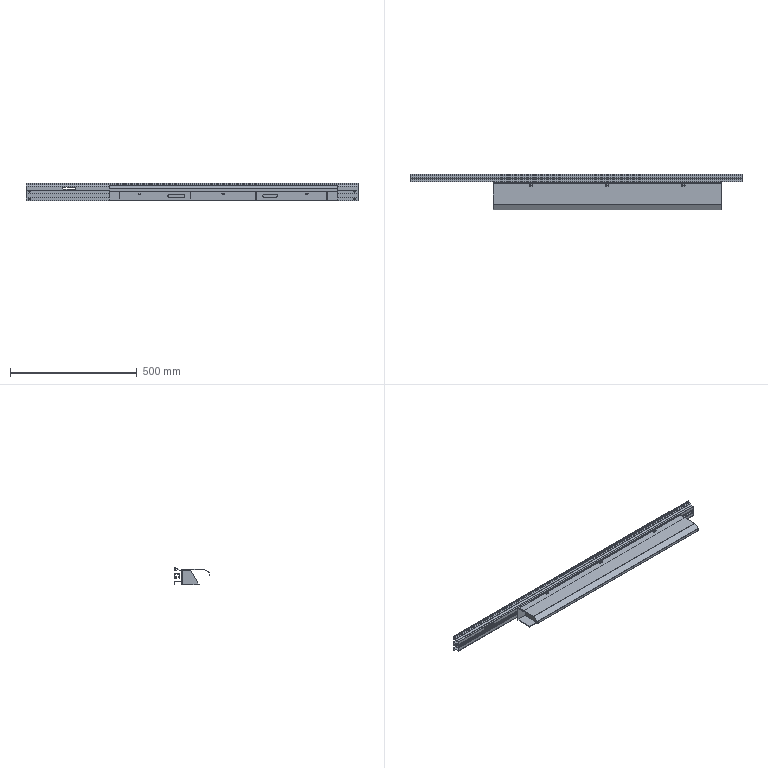Part | 7 solids | 256 faces | box 1310 x 141.151 x 70 mm | volume 1008218 mm3 | plane 168 | cylinder 88 | commonest cylinder face diameters 10 x21 6 x17 7 x12 9 x12 2 x9 3 x9